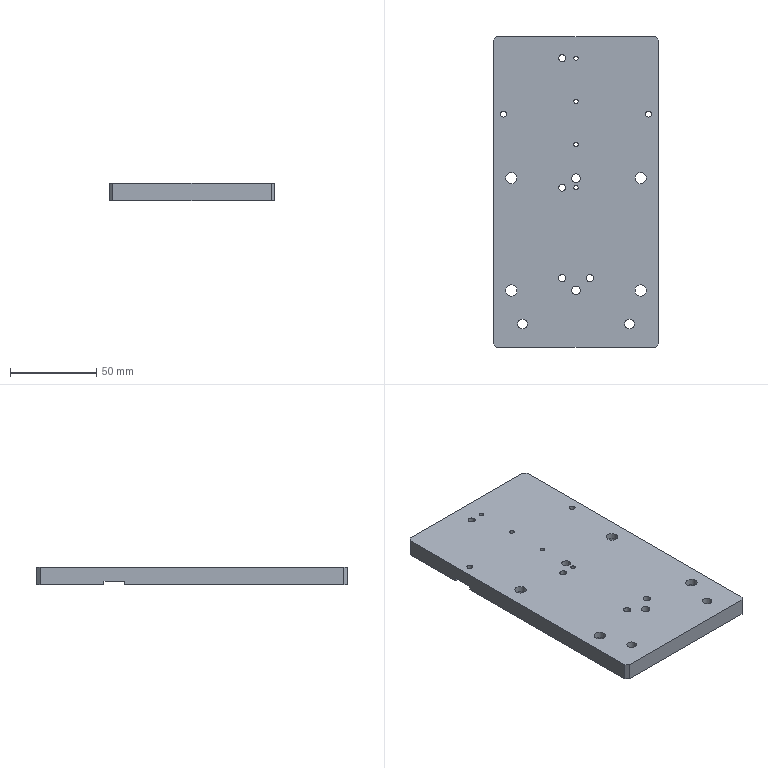Part | 1 solid | 44 faces | box 96 x 180 x 10 mm | volume 165169 mm3 | cylinder 24 | plane 20 | commonest cylinder face diameters 2.5 x4 6.6 x4 11 x4 3.3 x2 4 x2 4.2 x2
STEP:
#1=CARTESIAN_POINT('',(-32.,98.,6.4));
#2=VERTEX_POINT('',#1);
#3=CARTESIAN_POINT('',(-37.5,98.,6.4));
#4=DIRECTION('',(0.,0.,-1.));
#5=DIRECTION('',(1.,0.,0.));
#6=AXIS2_PLACEMENT_3D('',#3,#4,#5);
#7=CIRCLE('',#6,5.5);
#8=EDGE_CURVE('',#2,#2,#7,.T.);
#9=ORIENTED_EDGE('',*,*,#8,.T.);
#10=EDGE_LOOP('',(#9));
#11=FACE_BOUND('',#10,.T.);
#12=CARTESIAN_POINT('',(-34.2,98.,6.4));
#13=VERTEX_POINT('',#12);
#14=CARTESIAN_POINT('',(-37.5,98.,6.4));
#15=DIRECTION('',(0.,0.,-1.));
#16=DIRECTION('',(1.,0.,0.));
#17=AXIS2_PLACEMENT_3D('',#14,#15,#16);
#18=CIRCLE('',#17,3.3);
#19=EDGE_CURVE('',#13,#13,#18,.T.);
#20=ORIENTED_EDGE('',*,*,#19,.F.);
#21=EDGE_LOOP('',(#20));
#22=FACE_BOUND('',#21,.T.);
#23=CARTESIAN_POINT('',(-34.2,33.,6.4));
#24=DIRECTION('',(0.,0.,1.));
#25=DIRECTION('',(1.,0.,0.));
#26=AXIS2_PLACEMENT_3D('',#23,#24,#25);
#27=PLANE('',#26);
#28=ADVANCED_FACE('',(#11,#22),#27,.F.);
#29=CARTESIAN_POINT('',(43.,98.,6.4));
#30=VERTEX_POINT('',#29);
#31=CARTESIAN_POINT('',(37.5,98.,6.4));
#32=DIRECTION('',(0.,0.,-1.));
#33=DIRECTION('',(1.,0.,0.));
#34=AXIS2_PLACEMENT_3D('',#31,#32,#33);
#35=CIRCLE('',#34,5.5);
#36=EDGE_CURVE('',#30,#30,#35,.T.);
#37=ORIENTED_EDGE('',*,*,#36,.T.);
#38=EDGE_LOOP('',(#37));
#39=FACE_BOUND('',#38,.T.);
#40=CARTESIAN_POINT('',(40.8,98.,6.4));
#41=VERTEX_POINT('',#40);
#42=CARTESIAN_POINT('',(37.5,98.,6.4));
#43=DIRECTION('',(0.,0.,-1.));
#44=DIRECTION('',(1.,0.,0.));
#45=AXIS2_PLACEMENT_3D('',#42,#43,#44);
#46=CIRCLE('',#45,3.3);
#47=EDGE_CURVE('',#41,#41,#46,.T.);
#48=ORIENTED_EDGE('',*,*,#47,.F.);
#49=EDGE_LOOP('',(#48));
#50=FACE_BOUND('',#49,.T.);
#51=CARTESIAN_POINT('',(-34.2,33.,6.4));
#52=DIRECTION('',(0.,0.,1.));
#53=DIRECTION('',(1.,0.,0.));
#54=AXIS2_PLACEMENT_3D('',#51,#52,#53);
#55=PLANE('',#54);
#56=ADVANCED_FACE('',(#39,#50),#55,.F.);
#57=CARTESIAN_POINT('',(43.,33.,6.4));
#58=VERTEX_POINT('',#57);
#59=CARTESIAN_POINT('',(37.5,33.,6.4));
#60=DIRECTION('',(0.,0.,-1.));
#61=DIRECTION('',(1.,0.,0.));
#62=AXIS2_PLACEMENT_3D('',#59,#60,#61);
#63=CIRCLE('',#62,5.5);
#64=EDGE_CURVE('',#58,#58,#63,.T.);
#65=ORIENTED_EDGE('',*,*,#64,.T.);
#66=EDGE_LOOP('',(#65));
#67=FACE_BOUND('',#66,.T.);
#68=CARTESIAN_POINT('',(40.8,33.,6.4));
#69=VERTEX_POINT('',#68);
#70=CARTESIAN_POINT('',(37.5,33.,6.4));
#71=DIRECTION('',(0.,0.,-1.));
#72=DIRECTION('',(1.,0.,0.));
#73=AXIS2_PLACEMENT_3D('',#70,#71,#72);
#74=CIRCLE('',#73,3.3);
#75=EDGE_CURVE('',#69,#69,#74,.T.);
#76=ORIENTED_EDGE('',*,*,#75,.F.);
#77=EDGE_LOOP('',(#76));
#78=FACE_BOUND('',#77,.T.);
#79=CARTESIAN_POINT('',(-34.2,33.,6.4));
#80=DIRECTION('',(0.,0.,1.));
#81=DIRECTION('',(1.,0.,0.));
#82=AXIS2_PLACEMENT_3D('',#79,#80,#81);
#83=PLANE('',#82);
#84=ADVANCED_FACE('',(#67,#78),#83,.F.);
#85=CARTESIAN_POINT('',(-43.,33.,6.4));
#86=VERTEX_POINT('',#85);
#87=CARTESIAN_POINT('',(-37.5,33.,6.4));
#88=DIRECTION('',(0.,0.,-1.));
#89=DIRECTION('',(-1.,0.,0.));
#90=AXIS2_PLACEMENT_3D('',#87,#88,#89);
#91=CIRCLE('',#90,5.5);
#92=EDGE_CURVE('',#86,#86,#91,.T.);
#93=ORIENTED_EDGE('',*,*,#92,.T.);
#94=EDGE_LOOP('',(#93));
#95=FACE_BOUND('',#94,.T.);
#96=CARTESIAN_POINT('',(-40.8,33.,6.4));
#97=VERTEX_POINT('',#96);
#98=CARTESIAN_POINT('',(-37.5,33.,6.4));
#99=DIRECTION('',(0.,0.,-1.));
#100=DIRECTION('',(-1.,0.,0.));
#101=AXIS2_PLACEMENT_3D('',#98,#99,#100);
#102=CIRCLE('',#101,3.3);
#103=EDGE_CURVE('',#97,#97,#102,.T.);
#104=ORIENTED_EDGE('',*,*,#103,.F.);
#105=EDGE_LOOP('',(#104));
#106=FACE_BOUND('',#105,.T.);
#107=CARTESIAN_POINT('',(-34.2,33.,6.4));
#108=DIRECTION('',(0.,0.,1.));
#109=DIRECTION('',(1.,0.,0.));
#110=AXIS2_PLACEMENT_3D('',#107,#108,#109);
#111=PLANE('',#110);
#112=ADVANCED_FACE('',(#95,#106),#111,.F.);
#113=CARTESIAN_POINT('',(-48.,2.,10.));
#114=VERTEX_POINT('',#113);
#115=CARTESIAN_POINT('',(-46.,0.,10.));
#116=VERTEX_POINT('',#115);
#117=CARTESIAN_POINT('',(-46.,0.,10.));
#118=DIRECTION('',(0.7071,-0.7071,0.));
#119=VECTOR('',#118,1000.);
#120=LINE('',#117,#119);
#121=EDGE_CURVE('',#114,#116,#120,.T.);
#122=ORIENTED_EDGE('',*,*,#121,.F.);
#123=CARTESIAN_POINT('',(-48.,2.,0.));
#124=VERTEX_POINT('',#123);
#125=CARTESIAN_POINT('',(-48.,2.,10.));
#126=DIRECTION('',(0.,0.,1.));
#127=VECTOR('',#126,1000.);
#128=LINE('',#125,#127);
#129=EDGE_CURVE('',#124,#114,#128,.T.);
#130=ORIENTED_EDGE('',*,*,#129,.F.);
#131=CARTESIAN_POINT('',(-46.,0.,0.));
#132=VERTEX_POINT('',#131);
#133=CARTESIAN_POINT('',(-23.,-23.,0.));
#134=DIRECTION('',(-0.7071,0.7071,0.));
#135=VECTOR('',#134,1000.);
#136=LINE('',#133,#135);
#137=EDGE_CURVE('',#132,#124,#136,.T.);
#138=ORIENTED_EDGE('',*,*,#137,.F.);
#139=CARTESIAN_POINT('',(-46.,0.,10.));
#140=DIRECTION('',(0.,0.,-1.));
#141=VECTOR('',#140,1000.);
#142=LINE('',#139,#141);
#143=EDGE_CURVE('',#116,#132,#142,.T.);
#144=ORIENTED_EDGE('',*,*,#143,.F.);
#145=EDGE_LOOP('',(#122,#130,#138,#144));
#146=FACE_BOUND('',#145,.T.);
#147=CARTESIAN_POINT('',(-46.,0.,10.));
#148=DIRECTION('',(0.7071,0.7071,0.));
#149=DIRECTION('',(0.,0.,-1.));
#150=AXIS2_PLACEMENT_3D('',#147,#148,#149);
#151=PLANE('',#150);
#152=ADVANCED_FACE('',(#146),#151,.F.);
#153=CARTESIAN_POINT('',(46.,0.,10.));
#154=VERTEX_POINT('',#153);
#155=CARTESIAN_POINT('',(48.,2.,10.));
#156=VERTEX_POINT('',#155);
#157=CARTESIAN_POINT('',(48.,2.,10.));
#158=DIRECTION('',(0.7071,0.7071,0.));
#159=VECTOR('',#158,1000.);
#160=LINE('',#157,#159);
#161=EDGE_CURVE('',#154,#156,#160,.T.);
#162=ORIENTED_EDGE('',*,*,#161,.F.);
#163=CARTESIAN_POINT('',(46.,0.,0.));
#164=VERTEX_POINT('',#163);
#165=CARTESIAN_POINT('',(46.,0.,10.));
#166=DIRECTION('',(0.,0.,1.));
#167=VECTOR('',#166,1000.);
#168=LINE('',#165,#167);
#169=EDGE_CURVE('',#164,#154,#168,.T.);
#170=ORIENTED_EDGE('',*,*,#169,.F.);
#171=CARTESIAN_POINT('',(48.,2.,0.));
#172=VERTEX_POINT('',#171);
#173=CARTESIAN_POINT('',(23.,-23.,0.));
#174=DIRECTION('',(-0.7071,-0.7071,0.));
#175=VECTOR('',#174,1000.);
#176=LINE('',#173,#175);
#177=EDGE_CURVE('',#172,#164,#176,.T.);
#178=ORIENTED_EDGE('',*,*,#177,.F.);
#179=CARTESIAN_POINT('',(48.,2.,10.));
#180=DIRECTION('',(0.,0.,-1.));
#181=VECTOR('',#180,1000.);
#182=LINE('',#179,#181);
#183=EDGE_CURVE('',#156,#172,#182,.T.);
#184=ORIENTED_EDGE('',*,*,#183,.F.);
#185=EDGE_LOOP('',(#162,#170,#178,#184));
#186=FACE_BOUND('',#185,.T.);
#187=CARTESIAN_POINT('',(48.,2.,10.));
#188=DIRECTION('',(-0.7071,0.7071,0.));
#189=DIRECTION('',(0.,0.,-1.));
#190=AXIS2_PLACEMENT_3D('',#187,#188,#189);
#191=PLANE('',#190);
#192=ADVANCED_FACE('',(#186),#191,.F.);
#193=CARTESIAN_POINT('',(-46.,180.,10.));
#194=VERTEX_POINT('',#193);
#195=CARTESIAN_POINT('',(-48.,178.,10.));
#196=VERTEX_POINT('',#195);
#197=CARTESIAN_POINT('',(-48.,178.,10.));
#198=DIRECTION('',(-0.7071,-0.7071,0.));
#199=VECTOR('',#198,1000.);
#200=LINE('',#197,#199);
#201=EDGE_CURVE('',#194,#196,#200,.T.);
#202=ORIENTED_EDGE('',*,*,#201,.F.);
#203=CARTESIAN_POINT('',(-46.,180.,0.));
#204=VERTEX_POINT('',#203);
#205=CARTESIAN_POINT('',(-46.,180.,10.));
#206=DIRECTION('',(0.,0.,1.));
#207=VECTOR('',#206,1000.);
#208=LINE('',#205,#207);
#209=EDGE_CURVE('',#204,#194,#208,.T.);
#210=ORIENTED_EDGE('',*,*,#209,.F.);
#211=CARTESIAN_POINT('',(-48.,178.,0.));
#212=VERTEX_POINT('',#211);
#213=CARTESIAN_POINT('',(-113.,113.,0.));
#214=DIRECTION('',(0.7071,0.7071,0.));
#215=VECTOR('',#214,1000.);
#216=LINE('',#213,#215);
#217=EDGE_CURVE('',#212,#204,#216,.T.);
#218=ORIENTED_EDGE('',*,*,#217,.F.);
#219=CARTESIAN_POINT('',(-48.,178.,10.));
#220=DIRECTION('',(0.,0.,-1.));
#221=VECTOR('',#220,1000.);
#222=LINE('',#219,#221);
#223=EDGE_CURVE('',#196,#212,#222,.T.);
#224=ORIENTED_EDGE('',*,*,#223,.F.);
#225=EDGE_LOOP('',(#202,#210,#218,#224));
#226=FACE_BOUND('',#225,.T.);
#227=CARTESIAN_POINT('',(-48.,178.,10.));
#228=DIRECTION('',(0.7071,-0.7071,0.));
#229=DIRECTION('',(0.,0.,-1.));
#230=AXIS2_PLACEMENT_3D('',#227,#228,#229);
#231=PLANE('',#230);
#232=ADVANCED_FACE('',(#226),#231,.F.);
#233=CARTESIAN_POINT('',(48.,178.,10.));
#234=VERTEX_POINT('',#233);
#235=CARTESIAN_POINT('',(46.,180.,10.));
#236=VERTEX_POINT('',#235);
#237=CARTESIAN_POINT('',(46.,180.,10.));
#238=DIRECTION('',(-0.7071,0.7071,0.));
#239=VECTOR('',#238,1000.);
#240=LINE('',#237,#239);
#241=EDGE_CURVE('',#234,#236,#240,.T.);
#242=ORIENTED_EDGE('',*,*,#241,.F.);
#243=CARTESIAN_POINT('',(48.,178.,0.));
#244=VERTEX_POINT('',#243);
#245=CARTESIAN_POINT('',(48.,178.,10.));
#246=DIRECTION('',(0.,0.,1.));
#247=VECTOR('',#246,1000.);
#248=LINE('',#245,#247);
#249=EDGE_CURVE('',#244,#234,#248,.T.);
#250=ORIENTED_EDGE('',*,*,#249,.F.);
#251=CARTESIAN_POINT('',(46.,180.,0.));
#252=VERTEX_POINT('',#251);
#253=CARTESIAN_POINT('',(113.,113.,0.));
#254=DIRECTION('',(0.7071,-0.7071,0.));
#255=VECTOR('',#254,1000.);
#256=LINE('',#253,#255);
#257=EDGE_CURVE('',#252,#244,#256,.T.);
#258=ORIENTED_EDGE('',*,*,#257,.F.);
#259=CARTESIAN_POINT('',(46.,180.,10.));
#260=DIRECTION('',(0.,0.,-1.));
#261=VECTOR('',#260,1000.);
#262=LINE('',#259,#261);
#263=EDGE_CURVE('',#236,#252,#262,.T.);
#264=ORIENTED_EDGE('',*,*,#263,.F.);
#265=EDGE_LOOP('',(#242,#250,#258,#264));
#266=FACE_BOUND('',#265,.T.);
#267=CARTESIAN_POINT('',(46.,180.,10.));
#268=DIRECTION('',(-0.7071,-0.7071,0.));
#269=DIRECTION('',(0.,0.,-1.));
#270=AXIS2_PLACEMENT_3D('',#267,#268,#269);
#271=PLANE('',#270);
#272=ADVANCED_FACE('',(#266),#271,.F.);
#273=CARTESIAN_POINT('',(-26.,13.5,5.4));
#274=VERTEX_POINT('',#273);
#275=CARTESIAN_POINT('',(-31.,13.5,5.4));
#276=DIRECTION('',(0.,0.,-1.));
#277=DIRECTION('',(1.,0.,0.));
#278=AXIS2_PLACEMENT_3D('',#275,#276,#277);
#279=CIRCLE('',#278,5.);
#280=EDGE_CURVE('',#274,#274,#279,.T.);
#281=ORIENTED_EDGE('',*,*,#280,.T.);
#282=EDGE_LOOP('',(#281));
#283=FACE_BOUND('',#282,.T.);
#284=CARTESIAN_POINT('',(-28.25,13.5,5.4));
#285=VERTEX_POINT('',#284);
#286=CARTESIAN_POINT('',(-31.,13.5,5.4));
#287=DIRECTION('',(0.,0.,-1.));
#288=DIRECTION('',(1.,0.,0.));
#289=AXIS2_PLACEMENT_3D('',#286,#287,#288);
#290=CIRCLE('',#289,2.75);
#291=EDGE_CURVE('',#285,#285,#290,.T.);
#292=ORIENTED_EDGE('',*,*,#291,.F.);
#293=EDGE_LOOP('',(#292));
#294=FACE_BOUND('',#293,.T.);
#295=CARTESIAN_POINT('',(33.75,13.5,5.4));
#296=DIRECTION('',(0.,0.,1.));
#297=DIRECTION('',(1.,0.,0.));
#298=AXIS2_PLACEMENT_3D('',#295,#296,#297);
#299=PLANE('',#298);
#300=ADVANCED_FACE('',(#283,#294),#299,.F.);
#301=CARTESIAN_POINT('',(26.,13.5,5.4));
#302=VERTEX_POINT('',#301);
#303=CARTESIAN_POINT('',(31.,13.5,5.4));
#304=DIRECTION('',(0.,0.,-1.));
#305=DIRECTION('',(-1.,0.,0.));
#306=AXIS2_PLACEMENT_3D('',#303,#304,#305);
#307=CIRCLE('',#306,5.);
#308=EDGE_CURVE('',#302,#302,#307,.T.);
#309=ORIENTED_EDGE('',*,*,#308,.T.);
#310=EDGE_LOOP('',(#309));
#311=FACE_BOUND('',#310,.T.);
#312=CARTESIAN_POINT('',(28.25,13.5,5.4));
#313=VERTEX_POINT('',#312);
#314=CARTESIAN_POINT('',(31.,13.5,5.4));
#315=DIRECTION('',(0.,0.,-1.));
#316=DIRECTION('',(-1.,0.,0.));
#317=AXIS2_PLACEMENT_3D('',#314,#315,#316);
#318=CIRCLE('',#317,2.75);
#319=EDGE_CURVE('',#313,#313,#318,.T.);
#320=ORIENTED_EDGE('',*,*,#319,.F.);
#321=EDGE_LOOP('',(#320));
#322=FACE_BOUND('',#321,.T.);
#323=CARTESIAN_POINT('',(33.75,13.5,5.4));
#324=DIRECTION('',(0.,0.,1.));
#325=DIRECTION('',(1.,0.,0.));
#326=AXIS2_PLACEMENT_3D('',#323,#324,#325);
#327=PLANE('',#326);
#328=ADVANCED_FACE('',(#311,#322),#327,.F.);
#329=CARTESIAN_POINT('',(-48.,129.,2.));
#330=VERTEX_POINT('',#329);
#331=CARTESIAN_POINT('',(48.,129.,2.));
#332=VERTEX_POINT('',#331);
#333=CARTESIAN_POINT('',(-48.,129.,2.));
#334=DIRECTION('',(1.,0.,0.));
#335=VECTOR('',#334,1000.);
#336=LINE('',#333,#335);
#337=EDGE_CURVE('',#330,#332,#336,.T.);
#338=ORIENTED_EDGE('',*,*,#337,.F.);
#339=CARTESIAN_POINT('',(-48.,141.,2.));
#340=VERTEX_POINT('',#339);
#341=CARTESIAN_POINT('',(-48.,0.,2.));
#342=DIRECTION('',(0.,-1.,0.));
#343=VECTOR('',#342,1000.);
#344=LINE('',#341,#343);
#345=EDGE_CURVE('',#340,#330,#344,.T.);
#346=ORIENTED_EDGE('',*,*,#345,.F.);
#347=CARTESIAN_POINT('',(48.,141.,2.));
#348=VERTEX_POINT('',#347);
#349=CARTESIAN_POINT('',(0.,141.,2.));
#350=DIRECTION('',(1.,0.,0.));
#351=VECTOR('',#350,1000.);
#352=LINE('',#349,#351);
#353=EDGE_CURVE('',#340,#348,#352,.T.);
#354=ORIENTED_EDGE('',*,*,#353,.T.);
#355=CARTESIAN_POINT('',(48.,0.,2.));
#356=DIRECTION('',(0.,-1.,0.));
#357=VECTOR('',#356,1000.);
#358=LINE('',#355,#357);
#359=EDGE_CURVE('',#348,#332,#358,.T.);
#360=ORIENTED_EDGE('',*,*,#359,.T.);
#361=EDGE_LOOP('',(#338,#346,#354,#360));
#362=FACE_BOUND('',#361,.T.);
#363=CARTESIAN_POINT('',(-40.35,135.,2.));
#364=VERTEX_POINT('',#363);
#365=CARTESIAN_POINT('',(-42.,135.,2.));
#366=DIRECTION('',(0.,0.,1.));
#367=DIRECTION('',(1.,0.,0.));
#368=AXIS2_PLACEMENT_3D('',#365,#366,#367);
#369=CIRCLE('',#368,1.65);
#370=EDGE_CURVE('',#364,#364,#369,.T.);
#371=ORIENTED_EDGE('',*,*,#370,.T.);
#372=EDGE_LOOP('',(#371));
#373=FACE_BOUND('',#372,.T.);
#374=CARTESIAN_POINT('',(43.65,135.,2.));
#375=VERTEX_POINT('',#374);
#376=CARTESIAN_POINT('',(42.,135.,2.));
#377=DIRECTION('',(0.,0.,1.));
#378=DIRECTION('',(1.,0.,0.));
#379=AXIS2_PLACEMENT_3D('',#376,#377,#378);
#380=CIRCLE('',#379,1.65);
#381=EDGE_CURVE('',#375,#375,#380,.T.);
#382=ORIENTED_EDGE('',*,*,#381,.T.);
#383=EDGE_LOOP('',(#382));
#384=FACE_BOUND('',#383,.T.);
#385=CARTESIAN_POINT('',(0.,0.,2.));
#386=DIRECTION('',(0.,0.,1.));
#387=DIRECTION('',(1.,0.,0.));
#388=AXIS2_PLACEMENT_3D('',#385,#386,#387);
#389=PLANE('',#388);
#390=ADVANCED_FACE('',(#362,#373,#384),#389,.F.);
#391=CARTESIAN_POINT('',(48.,141.,0.));
#392=VERTEX_POINT('',#391);
#393=CARTESIAN_POINT('',(-48.,141.,0.));
#394=VERTEX_POINT('',#393);
#395=CARTESIAN_POINT('',(-48.,141.,0.));
#396=DIRECTION('',(-1.,0.,0.));
#397=VECTOR('',#396,1000.);
#398=LINE('',#395,#397);
#399=EDGE_CURVE('',#392,#394,#398,.T.);
#400=ORIENTED_EDGE('',*,*,#399,.F.);
#401=CARTESIAN_POINT('',(48.,141.,2.));
#402=DIRECTION('',(0.,0.,-1.));
#403=VECTOR('',#402,1000.);
#404=LINE('',#401,#403);
#405=EDGE_CURVE('',#348,#392,#404,.T.);
#406=ORIENTED_EDGE('',*,*,#405,.F.);
#407=ORIENTED_EDGE('',*,*,#353,.F.);
#408=CARTESIAN_POINT('',(-48.,141.,2.));
#409=DIRECTION('',(0.,0.,-1.));
#410=VECTOR('',#409,1000.);
#411=LINE('',#408,#410);
#412=EDGE_CURVE('',#340,#394,#411,.T.);
#413=ORIENTED_EDGE('',*,*,#412,.T.);
#414=EDGE_LOOP('',(#400,#406,#407,#413));
#415=FACE_BOUND('',#414,.T.);
#416=CARTESIAN_POINT('',(-48.,141.,2.));
#417=DIRECTION('',(0.,-1.,0.));
#418=DIRECTION('',(0.,0.,-1.));
#419=AXIS2_PLACEMENT_3D('',#416,#417,#418);
#420=PLANE('',#419);
#421=ADVANCED_FACE('',(#415),#420,.T.);
#422=CARTESIAN_POINT('',(-48.,129.,0.));
#423=VERTEX_POINT('',#422);
#424=CARTESIAN_POINT('',(48.,129.,0.));
#425=VERTEX_POINT('',#424);
#426=CARTESIAN_POINT('',(-48.,129.,0.));
#427=DIRECTION('',(1.,0.,0.));
#428=VECTOR('',#427,1000.);
#429=LINE('',#426,#428);
#430=EDGE_CURVE('',#423,#425,#429,.T.);
#431=ORIENTED_EDGE('',*,*,#430,.F.);
#432=CARTESIAN_POINT('',(-48.,129.,2.));
#433=DIRECTION('',(0.,0.,-1.));
#434=VECTOR('',#433,1000.);
#435=LINE('',#432,#434);
#436=EDGE_CURVE('',#330,#423,#435,.T.);
#437=ORIENTED_EDGE('',*,*,#436,.F.);
#438=ORIENTED_EDGE('',*,*,#337,.T.);
#439=CARTESIAN_POINT('',(48.,129.,2.));
#440=DIRECTION('',(0.,0.,-1.));
#441=VECTOR('',#440,1000.);
#442=LINE('',#439,#441);
#443=EDGE_CURVE('',#332,#425,#442,.T.);
#444=ORIENTED_EDGE('',*,*,#443,.T.);
#445=EDGE_LOOP('',(#431,#437,#438,#444));
#446=FACE_BOUND('',#445,.T.);
#447=CARTESIAN_POINT('',(-48.,129.,2.));
#448=DIRECTION('',(0.,1.,0.));
#449=DIRECTION('',(0.,0.,1.));
#450=AXIS2_PLACEMENT_3D('',#447,#448,#449);
#451=PLANE('',#450);
#452=ADVANCED_FACE('',(#446),#451,.T.);
#453=CARTESIAN_POINT('',(-1.25,92.5,10.));
#454=VERTEX_POINT('',#453);
#455=CARTESIAN_POINT('',(0.,92.5,10.));
#456=DIRECTION('',(0.,0.,-1.));
#457=DIRECTION('',(-1.,0.,0.));
#458=AXIS2_PLACEMENT_3D('',#455,#456,#457);
#459=CIRCLE('',#458,1.25);
#460=EDGE_CURVE('',#454,#454,#459,.T.);
#461=ORIENTED_EDGE('',*,*,#460,.T.);
#462=EDGE_LOOP('',(#461));
#463=FACE_BOUND('',#462,.T.);
#464=CARTESIAN_POINT('',(-1.25,117.5,10.));
#465=VERTEX_POINT('',#464);
#466=CARTESIAN_POINT('',(0.,117.5,10.));
#467=DIRECTION('',(0.,0.,-1.));
#468=DIRECTION('',(-1.,0.,0.));
#469=AXIS2_PLACEMENT_3D('',#466,#467,#468);
#470=CIRCLE('',#469,1.25);
#471=EDGE_CURVE('',#465,#465,#470,.T.);
#472=ORIENTED_EDGE('',*,*,#471,.T.);
#473=EDGE_LOOP('',(#472));
#474=FACE_BOUND('',#473,.T.);
#475=CARTESIAN_POINT('',(48.,0.,10.));
#476=DIRECTION('',(0.,1.,0.));
#477=VECTOR('',#476,1000.);
#478=LINE('',#475,#477);
#479=EDGE_CURVE('',#156,#234,#478,.T.);
#480=ORIENTED_EDGE('',*,*,#479,.T.);
#481=ORIENTED_EDGE('',*,*,#241,.T.);
#482=CARTESIAN_POINT('',(-48.,180.,10.));
#483=DIRECTION('',(-1.,0.,0.));
#484=VECTOR('',#483,1000.);
#485=LINE('',#482,#484);
#486=EDGE_CURVE('',#236,#194,#485,.T.);
#487=ORIENTED_EDGE('',*,*,#486,.T.);
#488=ORIENTED_EDGE('',*,*,#201,.T.);
#489=CARTESIAN_POINT('',(-48.,0.,10.));
#490=DIRECTION('',(0.,-1.,0.));
#491=VECTOR('',#490,1000.);
#492=LINE('',#489,#491);
#493=EDGE_CURVE('',#196,#114,#492,.T.);
#494=ORIENTED_EDGE('',*,*,#493,.T.);
#495=ORIENTED_EDGE('',*,*,#121,.T.);
#496=CARTESIAN_POINT('',(-48.,0.,10.));
#497=DIRECTION('',(1.,0.,0.));
#498=VECTOR('',#497,1000.);
#499=LINE('',#496,#498);
#500=EDGE_CURVE('',#116,#154,#499,.T.);
#501=ORIENTED_EDGE('',*,*,#500,.T.);
#502=ORIENTED_EDGE('',*,*,#161,.T.);
#503=EDGE_LOOP('',(#480,#481,#487,#488,#494,#495,#501,#502));
#504=FACE_BOUND('',#503,.T.);
#505=CARTESIAN_POINT('',(-1.25,167.5,10.));
#506=VERTEX_POINT('',#505);
#507=CARTESIAN_POINT('',(0.,167.5,10.));
#508=DIRECTION('',(0.,0.,-1.));
#509=DIRECTION('',(-1.,0.,0.));
#510=AXIS2_PLACEMENT_3D('',#507,#508,#509);
#511=CIRCLE('',#510,1.25);
#512=EDGE_CURVE('',#506,#506,#511,.T.);
#513=ORIENTED_EDGE('',*,*,#512,.T.);
#514=EDGE_LOOP('',(#513));
#515=FACE_BOUND('',#514,.T.);
#516=CARTESIAN_POINT('',(5.9,40.,10.));
#517=VERTEX_POINT('',#516);
#518=CARTESIAN_POINT('',(8.,40.,10.));
#519=DIRECTION('',(0.,0.,-1.));
#520=DIRECTION('',(-1.,0.,0.));
#521=AXIS2_PLACEMENT_3D('',#518,#519,#520);
#522=CIRCLE('',#521,2.1);
#523=EDGE_CURVE('',#517,#517,#522,.T.);
#524=ORIENTED_EDGE('',*,*,#523,.T.);
#525=EDGE_LOOP('',(#524));
#526=FACE_BOUND('',#525,.T.);
#527=CARTESIAN_POINT('',(-10.1,40.,10.));
#528=VERTEX_POINT('',#527);
#529=CARTESIAN_POINT('',(-8.,40.,10.));
#530=DIRECTION('',(0.,0.,-1.));
#531=DIRECTION('',(-1.,0.,0.));
#532=AXIS2_PLACEMENT_3D('',#529,#530,#531);
#533=CIRCLE('',#532,2.1);
#534=EDGE_CURVE('',#528,#528,#533,.T.);
#535=ORIENTED_EDGE('',*,*,#534,.T.);
#536=EDGE_LOOP('',(#535));
#537=FACE_BOUND('',#536,.T.);
#538=CARTESIAN_POINT('',(-1.25,142.5,10.));
#539=VERTEX_POINT('',#538);
#540=CARTESIAN_POINT('',(0.,142.5,10.));
#541=DIRECTION('',(0.,0.,-1.));
#542=DIRECTION('',(-1.,0.,0.));
#543=AXIS2_PLACEMENT_3D('',#540,#541,#542);
#544=CIRCLE('',#543,1.25);
#545=EDGE_CURVE('',#539,#539,#544,.T.);
#546=ORIENTED_EDGE('',*,*,#545,.T.);
#547=EDGE_LOOP('',(#546));
#548=FACE_BOUND('',#547,.T.);
#549=CARTESIAN_POINT('',(-10.,92.5,10.));
#550=VERTEX_POINT('',#549);
#551=CARTESIAN_POINT('',(-8.,92.5,10.));
#552=DIRECTION('',(0.,0.,-1.));
#553=DIRECTION('',(-1.,0.,0.));
#554=AXIS2_PLACEMENT_3D('',#551,#552,#553);
#555=CIRCLE('',#554,2.);
#556=EDGE_CURVE('',#550,#550,#555,.T.);
#557=ORIENTED_EDGE('',*,*,#556,.T.);
#558=EDGE_LOOP('',(#557));
#559=FACE_BOUND('',#558,.T.);
#560=CARTESIAN_POINT('',(-10.,167.5,10.));
#561=VERTEX_POINT('',#560);
#562=CARTESIAN_POINT('',(-8.,167.5,10.));
#563=DIRECTION('',(0.,0.,-1.));
#564=DIRECTION('',(-1.,0.,0.));
#565=AXIS2_PLACEMENT_3D('',#562,#563,#564);
#566=CIRCLE('',#565,2.);
#567=EDGE_CURVE('',#561,#561,#566,.T.);
#568=ORIENTED_EDGE('',*,*,#567,.T.);
#569=EDGE_LOOP('',(#568));
#570=FACE_BOUND('',#569,.T.);
#571=CARTESIAN_POINT('',(28.25,13.5,10.));
#572=VERTEX_POINT('',#571);
#573=CARTESIAN_POINT('',(31.,13.5,10.));
#574=DIRECTION('',(0.,0.,-1.));
#575=DIRECTION('',(-1.,0.,0.));
#576=AXIS2_PLACEMENT_3D('',#573,#574,#575);
#577=CIRCLE('',#576,2.75);
#578=EDGE_CURVE('',#572,#572,#577,.T.);
#579=ORIENTED_EDGE('',*,*,#578,.T.);
#580=EDGE_LOOP('',(#579));
#581=FACE_BOUND('',#580,.T.);
#582=CARTESIAN_POINT('',(-33.75,13.5,10.));
#583=VERTEX_POINT('',#582);
#584=CARTESIAN_POINT('',(-31.,13.5,10.));
#585=DIRECTION('',(0.,0.,-1.));
#586=DIRECTION('',(-1.,0.,0.));
#587=AXIS2_PLACEMENT_3D('',#584,#585,#586);
#588=CIRCLE('',#587,2.75);
#589=EDGE_CURVE('',#583,#583,#588,.T.);
#590=ORIENTED_EDGE('',*,*,#589,.T.);
#591=EDGE_LOOP('',(#590));
#592=FACE_BOUND('',#591,.T.);
#593=CARTESIAN_POINT('',(-43.65,135.,10.));
#594=VERTEX_POINT('',#593);
#595=CARTESIAN_POINT('',(-42.,135.,10.));
#596=DIRECTION('',(0.,0.,-1.));
#597=DIRECTION('',(-1.,0.,0.));
#598=AXIS2_PLACEMENT_3D('',#595,#596,#597);
#599=CIRCLE('',#598,1.65);
#600=EDGE_CURVE('',#594,#594,#599,.T.);
#601=ORIENTED_EDGE('',*,*,#600,.T.);
#602=EDGE_LOOP('',(#601));
#603=FACE_BOUND('',#602,.T.);
#604=CARTESIAN_POINT('',(40.35,135.,10.));
#605=VERTEX_POINT('',#604);
#606=CARTESIAN_POINT('',(42.,135.,10.));
#607=DIRECTION('',(0.,0.,-1.));
#608=DIRECTION('',(-1.,0.,0.));
#609=AXIS2_PLACEMENT_3D('',#606,#607,#608);
#610=CIRCLE('',#609,1.65);
#611=EDGE_CURVE('',#605,#605,#610,.T.);
#612=ORIENTED_EDGE('',*,*,#611,.T.);
#613=EDGE_LOOP('',(#612));
#614=FACE_BOUND('',#613,.T.);
#615=CARTESIAN_POINT('',(-40.8,33.,10.));
#616=VERTEX_POINT('',#615);
#617=CARTESIAN_POINT('',(-37.5,33.,10.));
#618=DIRECTION('',(0.,0.,-1.));
#619=DIRECTION('',(-1.,0.,0.));
#620=AXIS2_PLACEMENT_3D('',#617,#618,#619);
#621=CIRCLE('',#620,3.3);
#622=EDGE_CURVE('',#616,#616,#621,.T.);
#623=ORIENTED_EDGE('',*,*,#622,.T.);
#624=EDGE_LOOP('',(#623));
#625=FACE_BOUND('',#624,.T.);
#626=CARTESIAN_POINT('',(34.2,33.,10.));
#627=VERTEX_POINT('',#626);
#628=CARTESIAN_POINT('',(37.5,33.,10.));
#629=DIRECTION('',(0.,0.,-1.));
#630=DIRECTION('',(-1.,0.,0.));
#631=AXIS2_PLACEMENT_3D('',#628,#629,#630);
#632=CIRCLE('',#631,3.3);
#633=EDGE_CURVE('',#627,#627,#632,.T.);
#634=ORIENTED_EDGE('',*,*,#633,.T.);
#635=EDGE_LOOP('',(#634));
#636=FACE_BOUND('',#635,.T.);
#637=CARTESIAN_POINT('',(34.2,98.,10.));
#638=VERTEX_POINT('',#637);
#639=CARTESIAN_POINT('',(37.5,98.,10.));
#640=DIRECTION('',(0.,0.,-1.));
#641=DIRECTION('',(-1.,0.,0.));
#642=AXIS2_PLACEMENT_3D('',#639,#640,#641);
#643=CIRCLE('',#642,3.3);
#644=EDGE_CURVE('',#638,#638,#643,.T.);
#645=ORIENTED_EDGE('',*,*,#644,.T.);
#646=EDGE_LOOP('',(#645));
#647=FACE_BOUND('',#646,.T.);
#648=CARTESIAN_POINT('',(-40.8,98.,10.));
#649=VERTEX_POINT('',#648);
#650=CARTESIAN_POINT('',(-37.5,98.,10.));
#651=DIRECTION('',(0.,0.,-1.));
#652=DIRECTION('',(-1.,0.,0.));
#653=AXIS2_PLACEMENT_3D('',#650,#651,#652);
#654=CIRCLE('',#653,3.3);
#655=EDGE_CURVE('',#649,#649,#654,.T.);
#656=ORIENTED_EDGE('',*,*,#655,.T.);
#657=EDGE_LOOP('',(#656));
#658=FACE_BOUND('',#657,.T.);
#659=CARTESIAN_POINT('',(2.5,98.,10.));
#660=VERTEX_POINT('',#659);
#661=CARTESIAN_POINT('',(0.,98.,10.));
#662=DIRECTION('',(0.,0.,1.));
#663=DIRECTION('',(1.,0.,0.));
#664=AXIS2_PLACEMENT_3D('',#661,#662,#663);
#665=CIRCLE('',#664,2.5);
#666=EDGE_CURVE('',#660,#660,#665,.T.);
#667=ORIENTED_EDGE('',*,*,#666,.F.);
#668=EDGE_LOOP('',(#667));
#669=FACE_BOUND('',#668,.T.);
#670=CARTESIAN_POINT('',(2.5,33.,10.));
#671=VERTEX_POINT('',#670);
#672=CARTESIAN_POINT('',(0.,33.,10.));
#673=DIRECTION('',(0.,0.,1.));
#674=DIRECTION('',(1.,0.,0.));
#675=AXIS2_PLACEMENT_3D('',#672,#673,#674);
#676=CIRCLE('',#675,2.5);
#677=EDGE_CURVE('',#671,#671,#676,.T.);
#678=ORIENTED_EDGE('',*,*,#677,.F.);
#679=EDGE_LOOP('',(#678));
#680=FACE_BOUND('',#679,.T.);
#681=CARTESIAN_POINT('',(0.,0.,10.));
#682=DIRECTION('',(0.,0.,-1.));
#683=DIRECTION('',(-1.,0.,0.));
#684=AXIS2_PLACEMENT_3D('',#681,#682,#683);
#685=PLANE('',#684);
#686=ADVANCED_FACE('',(#463,#474,#504,#515,#526,#537,#548,#559,#570,#581,#592,#603,#614,#625,#636,#647,#658,#669,#680),#685,.F.);
#687=ORIENTED_EDGE('',*,*,#486,.F.);
#688=ORIENTED_EDGE('',*,*,#263,.T.);
#689=CARTESIAN_POINT('',(-48.,180.,0.));
#690=DIRECTION('',(-1.,0.,0.));
#691=VECTOR('',#690,1000.);
#692=LINE('',#689,#691);
#693=EDGE_CURVE('',#252,#204,#692,.T.);
#694=ORIENTED_EDGE('',*,*,#693,.T.);
#695=ORIENTED_EDGE('',*,*,#209,.T.);
#696=EDGE_LOOP('',(#687,#688,#694,#695));
#697=FACE_BOUND('',#696,.T.);
#698=CARTESIAN_POINT('',(-48.,180.,10.));
#699=DIRECTION('',(0.,-1.,0.));
#700=DIRECTION('',(0.,0.,-1.));
#701=AXIS2_PLACEMENT_3D('',#698,#699,#700);
#702=PLANE('',#701);
#703=ADVANCED_FACE('',(#697),#702,.F.);
#704=CARTESIAN_POINT('',(-48.,0.,0.));
#705=DIRECTION('',(1.,0.,0.));
#706=VECTOR('',#705,1000.);
#707=LINE('',#704,#706);
#708=EDGE_CURVE('',#132,#164,#707,.T.);
#709=ORIENTED_EDGE('',*,*,#708,.T.);
#710=ORIENTED_EDGE('',*,*,#169,.T.);
#711=ORIENTED_EDGE('',*,*,#500,.F.);
#712=ORIENTED_EDGE('',*,*,#143,.T.);
#713=EDGE_LOOP('',(#709,#710,#711,#712));
#714=FACE_BOUND('',#713,.T.);
#715=CARTESIAN_POINT('',(-48.,0.,10.));
#716=DIRECTION('',(0.,1.,0.));
#717=DIRECTION('',(0.,0.,1.));
#718=AXIS2_PLACEMENT_3D('',#715,#716,#717);
#719=PLANE('',#718);
#720=ADVANCED_FACE('',(#714),#719,.F.);
#721=ORIENTED_EDGE('',*,*,#693,.F.);
#722=ORIENTED_EDGE('',*,*,#257,.T.);
#723=CARTESIAN_POINT('',(48.,0.,0.));
#724=DIRECTION('',(0.,1.,0.));
#725=VECTOR('',#724,1000.);
#726=LINE('',#723,#725);
#727=EDGE_CURVE('',#392,#244,#726,.T.);
#728=ORIENTED_EDGE('',*,*,#727,.F.);
#729=ORIENTED_EDGE('',*,*,#399,.T.);
#730=CARTESIAN_POINT('',(-48.,0.,0.));
#731=DIRECTION('',(0.,-1.,0.));
#732=VECTOR('',#731,1000.);
#733=LINE('',#730,#732);
#734=EDGE_CURVE('',#212,#394,#733,.T.);
#735=ORIENTED_EDGE('',*,*,#734,.F.);
#736=ORIENTED_EDGE('',*,*,#217,.T.);
#737=EDGE_LOOP('',(#721,#722,#728,#729,#735,#736));
#738=FACE_BOUND('',#737,.T.);
#739=CARTESIAN_POINT('',(-10.,167.5,0.));
#740=VERTEX_POINT('',#739);
#741=CARTESIAN_POINT('',(-8.,167.5,0.));
#742=DIRECTION('',(0.,0.,-1.));
#743=DIRECTION('',(-1.,0.,0.));
#744=AXIS2_PLACEMENT_3D('',#741,#742,#743);
#745=CIRCLE('',#744,2.);
#746=EDGE_CURVE('',#740,#740,#745,.T.);
#747=ORIENTED_EDGE('',*,*,#746,.F.);
#748=EDGE_LOOP('',(#747));
#749=FACE_BOUND('',#748,.T.);
#750=CARTESIAN_POINT('',(-1.25,142.5,0.));
#751=VERTEX_POINT('',#750);
#752=CARTESIAN_POINT('',(0.,142.5,0.));
#753=DIRECTION('',(0.,0.,-1.));
#754=DIRECTION('',(-1.,0.,0.));
#755=AXIS2_PLACEMENT_3D('',#752,#753,#754);
#756=CIRCLE('',#755,1.25);
#757=EDGE_CURVE('',#751,#751,#756,.T.);
#758=ORIENTED_EDGE('',*,*,#757,.F.);
#759=EDGE_LOOP('',(#758));
#760=FACE_BOUND('',#759,.T.);
#761=CARTESIAN_POINT('',(-1.25,167.5,0.));
#762=VERTEX_POINT('',#761);
#763=CARTESIAN_POINT('',(0.,167.5,0.));
#764=DIRECTION('',(0.,0.,-1.));
#765=DIRECTION('',(-1.,0.,0.));
#766=AXIS2_PLACEMENT_3D('',#763,#764,#765);
#767=CIRCLE('',#766,1.25);
#768=EDGE_CURVE('',#762,#762,#767,.T.);
#769=ORIENTED_EDGE('',*,*,#768,.F.);
#770=EDGE_LOOP('',(#769));
#771=FACE_BOUND('',#770,.T.);
#772=CARTESIAN_POINT('',(0.,0.,0.));
#773=DIRECTION('',(0.,0.,-1.));
#774=DIRECTION('',(-1.,0.,0.));
#775=AXIS2_PLACEMENT_3D('',#772,#773,#774);
#776=PLANE('',#775);
#777=ADVANCED_FACE('',(#738,#749,#760,#771),#776,.T.);
#778=CARTESIAN_POINT('',(48.,0.,0.));
#779=DIRECTION('',(0.,1.,0.));
#780=VECTOR('',#779,1000.);
#781=LINE('',#778,#780);
#782=EDGE_CURVE('',#172,#425,#781,.T.);
#783=ORIENTED_EDGE('',*,*,#782,.F.);
#784=ORIENTED_EDGE('',*,*,#177,.T.);
#785=ORIENTED_EDGE('',*,*,#708,.F.);
#786=ORIENTED_EDGE('',*,*,#137,.T.);
#787=CARTESIAN_POINT('',(-48.,0.,0.));
#788=DIRECTION('',(0.,-1.,0.));
#789=VECTOR('',#788,1000.);
#790=LINE('',#787,#789);
#791=EDGE_CURVE('',#423,#124,#790,.T.);
#792=ORIENTED_EDGE('',*,*,#791,.F.);
#793=ORIENTED_EDGE('',*,*,#430,.T.);
#794=EDGE_LOOP('',(#783,#784,#785,#786,#792,#793));
#795=FACE_BOUND('',#794,.T.);
#796=CARTESIAN_POINT('',(-1.25,92.5,0.));
#797=VERTEX_POINT('',#796);
#798=CARTESIAN_POINT('',(0.,92.5,0.));
#799=DIRECTION('',(0.,0.,-1.));
#800=DIRECTION('',(-1.,0.,0.));
#801=AXIS2_PLACEMENT_3D('',#798,#799,#800);
#802=CIRCLE('',#801,1.25);
#803=EDGE_CURVE('',#797,#797,#802,.T.);
#804=ORIENTED_EDGE('',*,*,#803,.F.);
#805=EDGE_LOOP('',(#804));
#806=FACE_BOUND('',#805,.T.);
#807=CARTESIAN_POINT('',(-1.25,117.5,0.));
#808=VERTEX_POINT('',#807);
#809=CARTESIAN_POINT('',(0.,117.5,0.));
#810=DIRECTION('',(0.,0.,-1.));
#811=DIRECTION('',(-1.,0.,0.));
#812=AXIS2_PLACEMENT_3D('',#809,#810,#811);
#813=CIRCLE('',#812,1.25);
#814=EDGE_CURVE('',#808,#808,#813,.T.);
#815=ORIENTED_EDGE('',*,*,#814,.F.);
#816=EDGE_LOOP('',(#815));
#817=FACE_BOUND('',#816,.T.);
#818=CARTESIAN_POINT('',(5.9,40.,0.));
#819=VERTEX_POINT('',#818);
#820=CARTESIAN_POINT('',(8.,40.,0.));
#821=DIRECTION('',(0.,0.,-1.));
#822=DIRECTION('',(-1.,0.,0.));
#823=AXIS2_PLACEMENT_3D('',#820,#821,#822);
#824=CIRCLE('',#823,2.1);
#825=EDGE_CURVE('',#819,#819,#824,.T.);
#826=ORIENTED_EDGE('',*,*,#825,.F.);
#827=EDGE_LOOP('',(#826));
#828=FACE_BOUND('',#827,.T.);
#829=CARTESIAN_POINT('',(-10.1,40.,0.));
#830=VERTEX_POINT('',#829);
#831=CARTESIAN_POINT('',(-8.,40.,0.));
#832=DIRECTION('',(0.,0.,-1.));
#833=DIRECTION('',(-1.,0.,0.));
#834=AXIS2_PLACEMENT_3D('',#831,#832,#833);
#835=CIRCLE('',#834,2.1);
#836=EDGE_CURVE('',#830,#830,#835,.T.);
#837=ORIENTED_EDGE('',*,*,#836,.F.);
#838=EDGE_LOOP('',(#837));
#839=FACE_BOUND('',#838,.T.);
#840=CARTESIAN_POINT('',(-10.,92.5,0.));
#841=VERTEX_POINT('',#840);
#842=CARTESIAN_POINT('',(-8.,92.5,0.));
#843=DIRECTION('',(0.,0.,-1.));
#844=DIRECTION('',(-1.,0.,0.));
#845=AXIS2_PLACEMENT_3D('',#842,#843,#844);
#846=CIRCLE('',#845,2.);
#847=EDGE_CURVE('',#841,#841,#846,.T.);
#848=ORIENTED_EDGE('',*,*,#847,.F.);
#849=EDGE_LOOP('',(#848));
#850=FACE_BOUND('',#849,.T.);
#851=CARTESIAN_POINT('',(26.,13.5,0.));
#852=VERTEX_POINT('',#851);
#853=CARTESIAN_POINT('',(31.,13.5,0.));
#854=DIRECTION('',(0.,0.,-1.));
#855=DIRECTION('',(-1.,0.,0.));
#856=AXIS2_PLACEMENT_3D('',#853,#854,#855);
#857=CIRCLE('',#856,5.);
#858=EDGE_CURVE('',#852,#852,#857,.T.);
#859=ORIENTED_EDGE('',*,*,#858,.F.);
#860=EDGE_LOOP('',(#859));
#861=FACE_BOUND('',#860,.T.);
#862=CARTESIAN_POINT('',(-36.,13.5,0.));
#863=VERTEX_POINT('',#862);
#864=CARTESIAN_POINT('',(-31.,13.5,0.));
#865=DIRECTION('',(0.,0.,-1.));
#866=DIRECTION('',(-1.,0.,0.));
#867=AXIS2_PLACEMENT_3D('',#864,#865,#866);
#868=CIRCLE('',#867,5.);
#869=EDGE_CURVE('',#863,#863,#868,.T.);
#870=ORIENTED_EDGE('',*,*,#869,.F.);
#871=EDGE_LOOP('',(#870));
#872=FACE_BOUND('',#871,.T.);
#873=CARTESIAN_POINT('',(-43.,33.,0.));
#874=VERTEX_POINT('',#873);
#875=CARTESIAN_POINT('',(-37.5,33.,0.));
#876=DIRECTION('',(0.,0.,-1.));
#877=DIRECTION('',(-1.,0.,0.));
#878=AXIS2_PLACEMENT_3D('',#875,#876,#877);
#879=CIRCLE('',#878,5.5);
#880=EDGE_CURVE('',#874,#874,#879,.T.);
#881=ORIENTED_EDGE('',*,*,#880,.F.);
#882=EDGE_LOOP('',(#881));
#883=FACE_BOUND('',#882,.T.);
#884=CARTESIAN_POINT('',(32.,33.,0.));
#885=VERTEX_POINT('',#884);
#886=CARTESIAN_POINT('',(37.5,33.,0.));
#887=DIRECTION('',(0.,0.,-1.));
#888=DIRECTION('',(-1.,0.,0.));
#889=AXIS2_PLACEMENT_3D('',#886,#887,#888);
#890=CIRCLE('',#889,5.5);
#891=EDGE_CURVE('',#885,#885,#890,.T.);
#892=ORIENTED_EDGE('',*,*,#891,.F.);
#893=EDGE_LOOP('',(#892));
#894=FACE_BOUND('',#893,.T.);
#895=CARTESIAN_POINT('',(32.,98.,0.));
#896=VERTEX_POINT('',#895);
#897=CARTESIAN_POINT('',(37.5,98.,0.));
#898=DIRECTION('',(0.,0.,-1.));
#899=DIRECTION('',(-1.,0.,0.));
#900=AXIS2_PLACEMENT_3D('',#897,#898,#899);
#901=CIRCLE('',#900,5.5);
#902=EDGE_CURVE('',#896,#896,#901,.T.);
#903=ORIENTED_EDGE('',*,*,#902,.F.);
#904=EDGE_LOOP('',(#903));
#905=FACE_BOUND('',#904,.T.);
#906=CARTESIAN_POINT('',(-43.,98.,0.));
#907=VERTEX_POINT('',#906);
#908=CARTESIAN_POINT('',(-37.5,98.,0.));
#909=DIRECTION('',(0.,0.,-1.));
#910=DIRECTION('',(-1.,0.,0.));
#911=AXIS2_PLACEMENT_3D('',#908,#909,#910);
#912=CIRCLE('',#911,5.5);
#913=EDGE_CURVE('',#907,#907,#912,.T.);
#914=ORIENTED_EDGE('',*,*,#913,.F.);
#915=EDGE_LOOP('',(#914));
#916=FACE_BOUND('',#915,.T.);
#917=CARTESIAN_POINT('',(2.5,98.,0.));
#918=VERTEX_POINT('',#917);
#919=CARTESIAN_POINT('',(0.,98.,0.));
#920=DIRECTION('',(0.,0.,1.));
#921=DIRECTION('',(1.,0.,0.));
#922=AXIS2_PLACEMENT_3D('',#919,#920,#921);
#923=CIRCLE('',#922,2.5);
#924=EDGE_CURVE('',#918,#918,#923,.T.);
#925=ORIENTED_EDGE('',*,*,#924,.T.);
#926=EDGE_LOOP('',(#925));
#927=FACE_BOUND('',#926,.T.);
#928=CARTESIAN_POINT('',(2.5,33.,0.));
#929=VERTEX_POINT('',#928);
#930=CARTESIAN_POINT('',(0.,33.,0.));
#931=DIRECTION('',(0.,0.,1.));
#932=DIRECTION('',(1.,0.,0.));
#933=AXIS2_PLACEMENT_3D('',#930,#931,#932);
#934=CIRCLE('',#933,2.5);
#935=EDGE_CURVE('',#929,#929,#934,.T.);
#936=ORIENTED_EDGE('',*,*,#935,.T.);
#937=EDGE_LOOP('',(#936));
#938=FACE_BOUND('',#937,.T.);
#939=CARTESIAN_POINT('',(0.,0.,0.));
#940=DIRECTION('',(0.,0.,-1.));
#941=DIRECTION('',(-1.,0.,0.));
#942=AXIS2_PLACEMENT_3D('',#939,#940,#941);
#943=PLANE('',#942);
#944=ADVANCED_FACE('',(#795,#806,#817,#828,#839,#850,#861,#872,#883,#894,#905,#916,#927,#938),#943,.T.);
#945=ORIENTED_EDGE('',*,*,#727,.T.);
#946=ORIENTED_EDGE('',*,*,#249,.T.);
#947=ORIENTED_EDGE('',*,*,#479,.F.);
#948=ORIENTED_EDGE('',*,*,#183,.T.);
#949=ORIENTED_EDGE('',*,*,#782,.T.);
#950=ORIENTED_EDGE('',*,*,#443,.F.);
#951=ORIENTED_EDGE('',*,*,#359,.F.);
#952=ORIENTED_EDGE('',*,*,#405,.T.);
#953=EDGE_LOOP('',(#945,#946,#947,#948,#949,#950,#951,#952));
#954=FACE_BOUND('',#953,.T.);
#955=CARTESIAN_POINT('',(48.,0.,10.));
#956=DIRECTION('',(-1.,0.,0.));
#957=DIRECTION('',(0.,0.,1.));
#958=AXIS2_PLACEMENT_3D('',#955,#956,#957);
#959=PLANE('',#958);
#960=ADVANCED_FACE('',(#954),#959,.F.);
#961=ORIENTED_EDGE('',*,*,#493,.F.);
#962=ORIENTED_EDGE('',*,*,#223,.T.);
#963=ORIENTED_EDGE('',*,*,#734,.T.);
#964=ORIENTED_EDGE('',*,*,#412,.F.);
#965=ORIENTED_EDGE('',*,*,#345,.T.);
#966=ORIENTED_EDGE('',*,*,#436,.T.);
#967=ORIENTED_EDGE('',*,*,#791,.T.);
#968=ORIENTED_EDGE('',*,*,#129,.T.);
#969=EDGE_LOOP('',(#961,#962,#963,#964,#965,#966,#967,#968));
#970=FACE_BOUND('',#969,.T.);
#971=CARTESIAN_POINT('',(-48.,0.,10.));
#972=DIRECTION('',(1.,0.,0.));
#973=DIRECTION('',(0.,0.,-1.));
#974=AXIS2_PLACEMENT_3D('',#971,#972,#973);
#975=PLANE('',#974);
#976=ADVANCED_FACE('',(#970),#975,.F.);
#977=ORIENTED_EDGE('',*,*,#803,.T.);
#978=EDGE_LOOP('',(#977));
#979=FACE_BOUND('',#978,.T.);
#980=ORIENTED_EDGE('',*,*,#460,.F.);
#981=EDGE_LOOP('',(#980));
#982=FACE_BOUND('',#981,.T.);
#983=CARTESIAN_POINT('',(0.,92.5,0.));
#984=DIRECTION('',(0.,0.,-1.));
#985=DIRECTION('',(-1.,0.,0.));
#986=AXIS2_PLACEMENT_3D('',#983,#984,#985);
#987=CYLINDRICAL_SURFACE('',#986,1.25);
#988=ADVANCED_FACE('',(#979,#982),#987,.F.);
#989=ORIENTED_EDGE('',*,*,#814,.T.);
#990=EDGE_LOOP('',(#989));
#991=FACE_BOUND('',#990,.T.);
#992=ORIENTED_EDGE('',*,*,#471,.F.);
#993=EDGE_LOOP('',(#992));
#994=FACE_BOUND('',#993,.T.);
#995=CARTESIAN_POINT('',(0.,117.5,0.));
#996=DIRECTION('',(0.,0.,-1.));
#997=DIRECTION('',(-1.,0.,0.));
#998=AXIS2_PLACEMENT_3D('',#995,#996,#997);
#999=CYLINDRICAL_SURFACE('',#998,1.25);
#1000=ADVANCED_FACE('',(#991,#994),#999,.F.);
#1001=ORIENTED_EDGE('',*,*,#768,.T.);
#1002=EDGE_LOOP('',(#1001));
#1003=FACE_BOUND('',#1002,.T.);
#1004=ORIENTED_EDGE('',*,*,#512,.F.);
#1005=EDGE_LOOP('',(#1004));
#1006=FACE_BOUND('',#1005,.T.);
#1007=CARTESIAN_POINT('',(0.,167.5,0.));
#1008=DIRECTION('',(0.,0.,-1.));
#1009=DIRECTION('',(-1.,0.,0.));
#1010=AXIS2_PLACEMENT_3D('',#1007,#1008,#1009);
#1011=CYLINDRICAL_SURFACE('',#1010,1.25);
#1012=ADVANCED_FACE('',(#1003,#1006),#1011,.F.);
#1013=ORIENTED_EDGE('',*,*,#825,.T.);
#1014=EDGE_LOOP('',(#1013));
#1015=FACE_BOUND('',#1014,.T.);
#1016=ORIENTED_EDGE('',*,*,#523,.F.);
#1017=EDGE_LOOP('',(#1016));
#1018=FACE_BOUND('',#1017,.T.);
#1019=CARTESIAN_POINT('',(8.,40.,0.));
#1020=DIRECTION('',(0.,0.,-1.));
#1021=DIRECTION('',(-1.,0.,0.));
#1022=AXIS2_PLACEMENT_3D('',#1019,#1020,#1021);
#1023=CYLINDRICAL_SURFACE('',#1022,2.1);
#1024=ADVANCED_FACE('',(#1015,#1018),#1023,.F.);
#1025=ORIENTED_EDGE('',*,*,#836,.T.);
#1026=EDGE_LOOP('',(#1025));
#1027=FACE_BOUND('',#1026,.T.);
#1028=ORIENTED_EDGE('',*,*,#534,.F.);
#1029=EDGE_LOOP('',(#1028));
#1030=FACE_BOUND('',#1029,.T.);
#1031=CARTESIAN_POINT('',(-8.,40.,0.));
#1032=DIRECTION('',(0.,0.,-1.));
#1033=DIRECTION('',(-1.,0.,0.));
#1034=AXIS2_PLACEMENT_3D('',#1031,#1032,#1033);
#1035=CYLINDRICAL_SURFACE('',#1034,2.1);
#1036=ADVANCED_FACE('',(#1027,#1030),#1035,.F.);
#1037=ORIENTED_EDGE('',*,*,#757,.T.);
#1038=EDGE_LOOP('',(#1037));
#1039=FACE_BOUND('',#1038,.T.);
#1040=ORIENTED_EDGE('',*,*,#545,.F.);
#1041=EDGE_LOOP('',(#1040));
#1042=FACE_BOUND('',#1041,.T.);
#1043=CARTESIAN_POINT('',(0.,142.5,0.));
#1044=DIRECTION('',(0.,0.,-1.));
#1045=DIRECTION('',(-1.,0.,0.));
#1046=AXIS2_PLACEMENT_3D('',#1043,#1044,#1045);
#1047=CYLINDRICAL_SURFACE('',#1046,1.25);
#1048=ADVANCED_FACE('',(#1039,#1042),#1047,.F.);
#1049=ORIENTED_EDGE('',*,*,#847,.T.);
#1050=EDGE_LOOP('',(#1049));
#1051=FACE_BOUND('',#1050,.T.);
#1052=ORIENTED_EDGE('',*,*,#556,.F.);
#1053=EDGE_LOOP('',(#1052));
#1054=FACE_BOUND('',#1053,.T.);
#1055=CARTESIAN_POINT('',(-8.,92.5,0.));
#1056=DIRECTION('',(0.,0.,-1.));
#1057=DIRECTION('',(-1.,0.,0.));
#1058=AXIS2_PLACEMENT_3D('',#1055,#1056,#1057);
#1059=CYLINDRICAL_SURFACE('',#1058,2.);
#1060=ADVANCED_FACE('',(#1051,#1054),#1059,.F.);
#1061=ORIENTED_EDGE('',*,*,#746,.T.);
#1062=EDGE_LOOP('',(#1061));
#1063=FACE_BOUND('',#1062,.T.);
#1064=ORIENTED_EDGE('',*,*,#567,.F.);
#1065=EDGE_LOOP('',(#1064));
#1066=FACE_BOUND('',#1065,.T.);
#1067=CARTESIAN_POINT('',(-8.,167.5,0.));
#1068=DIRECTION('',(0.,0.,-1.));
#1069=DIRECTION('',(-1.,0.,0.));
#1070=AXIS2_PLACEMENT_3D('',#1067,#1068,#1069);
#1071=CYLINDRICAL_SURFACE('',#1070,2.);
#1072=ADVANCED_FACE('',(#1063,#1066),#1071,.F.);
#1073=ORIENTED_EDGE('',*,*,#319,.T.);
#1074=EDGE_LOOP('',(#1073));
#1075=FACE_BOUND('',#1074,.T.);
#1076=ORIENTED_EDGE('',*,*,#578,.F.);
#1077=EDGE_LOOP('',(#1076));
#1078=FACE_BOUND('',#1077,.T.);
#1079=CARTESIAN_POINT('',(31.,13.5,0.));
#1080=DIRECTION('',(0.,0.,-1.));
#1081=DIRECTION('',(-1.,0.,0.));
#1082=AXIS2_PLACEMENT_3D('',#1079,#1080,#1081);
#1083=CYLINDRICAL_SURFACE('',#1082,2.75);
#1084=ADVANCED_FACE('',(#1075,#1078),#1083,.F.);
#1085=ORIENTED_EDGE('',*,*,#858,.T.);
#1086=EDGE_LOOP('',(#1085));
#1087=FACE_BOUND('',#1086,.T.);
#1088=ORIENTED_EDGE('',*,*,#308,.F.);
#1089=EDGE_LOOP('',(#1088));
#1090=FACE_BOUND('',#1089,.T.);
#1091=CARTESIAN_POINT('',(31.,13.5,0.));
#1092=DIRECTION('',(0.,0.,-1.));
#1093=DIRECTION('',(-1.,0.,0.));
#1094=AXIS2_PLACEMENT_3D('',#1091,#1092,#1093);
#1095=CYLINDRICAL_SURFACE('',#1094,5.);
#1096=ADVANCED_FACE('',(#1087,#1090),#1095,.F.);
#1097=ORIENTED_EDGE('',*,*,#291,.T.);
#1098=EDGE_LOOP('',(#1097));
#1099=FACE_BOUND('',#1098,.T.);
#1100=ORIENTED_EDGE('',*,*,#589,.F.);
#1101=EDGE_LOOP('',(#1100));
#1102=FACE_BOUND('',#1101,.T.);
#1103=CARTESIAN_POINT('',(-31.,13.5,0.));
#1104=DIRECTION('',(0.,0.,-1.));
#1105=DIRECTION('',(-1.,0.,0.));
#1106=AXIS2_PLACEMENT_3D('',#1103,#1104,#1105);
#1107=CYLINDRICAL_SURFACE('',#1106,2.75);
#1108=ADVANCED_FACE('',(#1099,#1102),#1107,.F.);
#1109=ORIENTED_EDGE('',*,*,#869,.T.);
#1110=EDGE_LOOP('',(#1109));
#1111=FACE_BOUND('',#1110,.T.);
#1112=ORIENTED_EDGE('',*,*,#280,.F.);
#1113=EDGE_LOOP('',(#1112));
#1114=FACE_BOUND('',#1113,.T.);
#1115=CARTESIAN_POINT('',(-31.,13.5,0.));
#1116=DIRECTION('',(0.,0.,-1.));
#1117=DIRECTION('',(-1.,0.,0.));
#1118=AXIS2_PLACEMENT_3D('',#1115,#1116,#1117);
#1119=CYLINDRICAL_SURFACE('',#1118,5.);
#1120=ADVANCED_FACE('',(#1111,#1114),#1119,.F.);
#1121=ORIENTED_EDGE('',*,*,#370,.F.);
#1122=EDGE_LOOP('',(#1121));
#1123=FACE_BOUND('',#1122,.T.);
#1124=ORIENTED_EDGE('',*,*,#600,.F.);
#1125=EDGE_LOOP('',(#1124));
#1126=FACE_BOUND('',#1125,.T.);
#1127=CARTESIAN_POINT('',(-42.,135.,0.));
#1128=DIRECTION('',(0.,0.,-1.));
#1129=DIRECTION('',(-1.,0.,0.));
#1130=AXIS2_PLACEMENT_3D('',#1127,#1128,#1129);
#1131=CYLINDRICAL_SURFACE('',#1130,1.65);
#1132=ADVANCED_FACE('',(#1123,#1126),#1131,.F.);
#1133=ORIENTED_EDGE('',*,*,#381,.F.);
#1134=EDGE_LOOP('',(#1133));
#1135=FACE_BOUND('',#1134,.T.);
#1136=ORIENTED_EDGE('',*,*,#611,.F.);
#1137=EDGE_LOOP('',(#1136));
#1138=FACE_BOUND('',#1137,.T.);
#1139=CARTESIAN_POINT('',(42.,135.,0.));
#1140=DIRECTION('',(0.,0.,-1.));
#1141=DIRECTION('',(-1.,0.,0.));
#1142=AXIS2_PLACEMENT_3D('',#1139,#1140,#1141);
#1143=CYLINDRICAL_SURFACE('',#1142,1.65);
#1144=ADVANCED_FACE('',(#1135,#1138),#1143,.F.);
#1145=ORIENTED_EDGE('',*,*,#103,.T.);
#1146=EDGE_LOOP('',(#1145));
#1147=FACE_BOUND('',#1146,.T.);
#1148=ORIENTED_EDGE('',*,*,#622,.F.);
#1149=EDGE_LOOP('',(#1148));
#1150=FACE_BOUND('',#1149,.T.);
#1151=CARTESIAN_POINT('',(-37.5,33.,0.));
#1152=DIRECTION('',(0.,0.,-1.));
#1153=DIRECTION('',(-1.,0.,0.));
#1154=AXIS2_PLACEMENT_3D('',#1151,#1152,#1153);
#1155=CYLINDRICAL_SURFACE('',#1154,3.3);
#1156=ADVANCED_FACE('',(#1147,#1150),#1155,.F.);
#1157=ORIENTED_EDGE('',*,*,#880,.T.);
#1158=EDGE_LOOP('',(#1157));
#1159=FACE_BOUND('',#1158,.T.);
#1160=ORIENTED_EDGE('',*,*,#92,.F.);
#1161=EDGE_LOOP('',(#1160));
#1162=FACE_BOUND('',#1161,.T.);
#1163=CARTESIAN_POINT('',(-37.5,33.,0.));
#1164=DIRECTION('',(0.,0.,-1.));
#1165=DIRECTION('',(-1.,0.,0.));
#1166=AXIS2_PLACEMENT_3D('',#1163,#1164,#1165);
#1167=CYLINDRICAL_SURFACE('',#1166,5.5);
#1168=ADVANCED_FACE('',(#1159,#1162),#1167,.F.);
#1169=ORIENTED_EDGE('',*,*,#75,.T.);
#1170=EDGE_LOOP('',(#1169));
#1171=FACE_BOUND('',#1170,.T.);
#1172=ORIENTED_EDGE('',*,*,#633,.F.);
#1173=EDGE_LOOP('',(#1172));
#1174=FACE_BOUND('',#1173,.T.);
#1175=CARTESIAN_POINT('',(37.5,33.,0.));
#1176=DIRECTION('',(0.,0.,-1.));
#1177=DIRECTION('',(-1.,0.,0.));
#1178=AXIS2_PLACEMENT_3D('',#1175,#1176,#1177);
#1179=CYLINDRICAL_SURFACE('',#1178,3.3);
#1180=ADVANCED_FACE('',(#1171,#1174),#1179,.F.);
#1181=ORIENTED_EDGE('',*,*,#891,.T.);
#1182=EDGE_LOOP('',(#1181));
#1183=FACE_BOUND('',#1182,.T.);
#1184=ORIENTED_EDGE('',*,*,#64,.F.);
#1185=EDGE_LOOP('',(#1184));
#1186=FACE_BOUND('',#1185,.T.);
#1187=CARTESIAN_POINT('',(37.5,33.,0.));
#1188=DIRECTION('',(0.,0.,-1.));
#1189=DIRECTION('',(-1.,0.,0.));
#1190=AXIS2_PLACEMENT_3D('',#1187,#1188,#1189);
#1191=CYLINDRICAL_SURFACE('',#1190,5.5);
#1192=ADVANCED_FACE('',(#1183,#1186),#1191,.F.);
#1193=ORIENTED_EDGE('',*,*,#47,.T.);
#1194=EDGE_LOOP('',(#1193));
#1195=FACE_BOUND('',#1194,.T.);
#1196=ORIENTED_EDGE('',*,*,#644,.F.);
#1197=EDGE_LOOP('',(#1196));
#1198=FACE_BOUND('',#1197,.T.);
#1199=CARTESIAN_POINT('',(37.5,98.,0.));
#1200=DIRECTION('',(0.,0.,-1.));
#1201=DIRECTION('',(-1.,0.,0.));
#1202=AXIS2_PLACEMENT_3D('',#1199,#1200,#1201);
#1203=CYLINDRICAL_SURFACE('',#1202,3.3);
#1204=ADVANCED_FACE('',(#1195,#1198),#1203,.F.);
#1205=ORIENTED_EDGE('',*,*,#902,.T.);
#1206=EDGE_LOOP('',(#1205));
#1207=FACE_BOUND('',#1206,.T.);
#1208=ORIENTED_EDGE('',*,*,#36,.F.);
#1209=EDGE_LOOP('',(#1208));
#1210=FACE_BOUND('',#1209,.T.);
#1211=CARTESIAN_POINT('',(37.5,98.,0.));
#1212=DIRECTION('',(0.,0.,-1.));
#1213=DIRECTION('',(-1.,0.,0.));
#1214=AXIS2_PLACEMENT_3D('',#1211,#1212,#1213);
#1215=CYLINDRICAL_SURFACE('',#1214,5.5);
#1216=ADVANCED_FACE('',(#1207,#1210),#1215,.F.);
#1217=ORIENTED_EDGE('',*,*,#19,.T.);
#1218=EDGE_LOOP('',(#1217));
#1219=FACE_BOUND('',#1218,.T.);
#1220=ORIENTED_EDGE('',*,*,#655,.F.);
#1221=EDGE_LOOP('',(#1220));
#1222=FACE_BOUND('',#1221,.T.);
#1223=CARTESIAN_POINT('',(-37.5,98.,0.));
#1224=DIRECTION('',(0.,0.,-1.));
#1225=DIRECTION('',(-1.,0.,0.));
#1226=AXIS2_PLACEMENT_3D('',#1223,#1224,#1225);
#1227=CYLINDRICAL_SURFACE('',#1226,3.3);
#1228=ADVANCED_FACE('',(#1219,#1222),#1227,.F.);
#1229=ORIENTED_EDGE('',*,*,#913,.T.);
#1230=EDGE_LOOP('',(#1229));
#1231=FACE_BOUND('',#1230,.T.);
#1232=ORIENTED_EDGE('',*,*,#8,.F.);
#1233=EDGE_LOOP('',(#1232));
#1234=FACE_BOUND('',#1233,.T.);
#1235=CARTESIAN_POINT('',(-37.5,98.,0.));
#1236=DIRECTION('',(0.,0.,-1.));
#1237=DIRECTION('',(-1.,0.,0.));
#1238=AXIS2_PLACEMENT_3D('',#1235,#1236,#1237);
#1239=CYLINDRICAL_SURFACE('',#1238,5.5);
#1240=ADVANCED_FACE('',(#1231,#1234),#1239,.F.);
#1241=ORIENTED_EDGE('',*,*,#924,.F.);
#1242=EDGE_LOOP('',(#1241));
#1243=FACE_BOUND('',#1242,.T.);
#1244=ORIENTED_EDGE('',*,*,#666,.T.);
#1245=EDGE_LOOP('',(#1244));
#1246=FACE_BOUND('',#1245,.T.);
#1247=CARTESIAN_POINT('',(0.,98.,10.));
#1248=DIRECTION('',(0.,0.,1.));
#1249=DIRECTION('',(1.,0.,0.));
#1250=AXIS2_PLACEMENT_3D('',#1247,#1248,#1249);
#1251=CYLINDRICAL_SURFACE('',#1250,2.5);
#1252=ADVANCED_FACE('',(#1243,#1246),#1251,.F.);
#1253=ORIENTED_EDGE('',*,*,#935,.F.);
#1254=EDGE_LOOP('',(#1253));
#1255=FACE_BOUND('',#1254,.T.);
#1256=ORIENTED_EDGE('',*,*,#677,.T.);
#1257=EDGE_LOOP('',(#1256));
#1258=FACE_BOUND('',#1257,.T.);
#1259=CARTESIAN_POINT('',(0.,33.,10.));
#1260=DIRECTION('',(0.,0.,1.));
#1261=DIRECTION('',(1.,0.,0.));
#1262=AXIS2_PLACEMENT_3D('',#1259,#1260,#1261);
#1263=CYLINDRICAL_SURFACE('',#1262,2.5);
#1264=ADVANCED_FACE('',(#1255,#1258),#1263,.F.);
#1265=CLOSED_SHELL('',(#28,#56,#84,#112,#152,#192,#232,#272,#300,#328,#390,#421,#452,#686,#703,#720,#777,#944,#960,#976,#988,#1000,#1012,#1024,#1036,#1048,#1060,#1072,#1084,#1096,#1108,#1120,#1132,#1144,#1156,#1168,#1180,#1192,#1204,#1216,#1228,#1240,#1252,#1264));
#1266=MANIFOLD_SOLID_BREP('',#1265);
#1267=(LENGTH_UNIT()NAMED_UNIT(*)SI_UNIT(.MILLI.,.METRE.));
#1268=UNCERTAINTY_MEASURE_WITH_UNIT(LENGTH_MEASURE(0.00001),#1267,'','');
#1269=(NAMED_UNIT(*)PLANE_ANGLE_UNIT()SI_UNIT($,.RADIAN.));
#1270=(NAMED_UNIT(*)SI_UNIT($,.STERADIAN.)SOLID_ANGLE_UNIT());
#1271=(GEOMETRIC_REPRESENTATION_CONTEXT(3)GLOBAL_UNCERTAINTY_ASSIGNED_CONTEXT((#1268))GLOBAL_UNIT_ASSIGNED_CONTEXT((#1267,#1269,#1270))REPRESENTATION_CONTEXT('',''));
#1272=ADVANCED_BREP_SHAPE_REPRESENTATION('',(#1266),#1271);